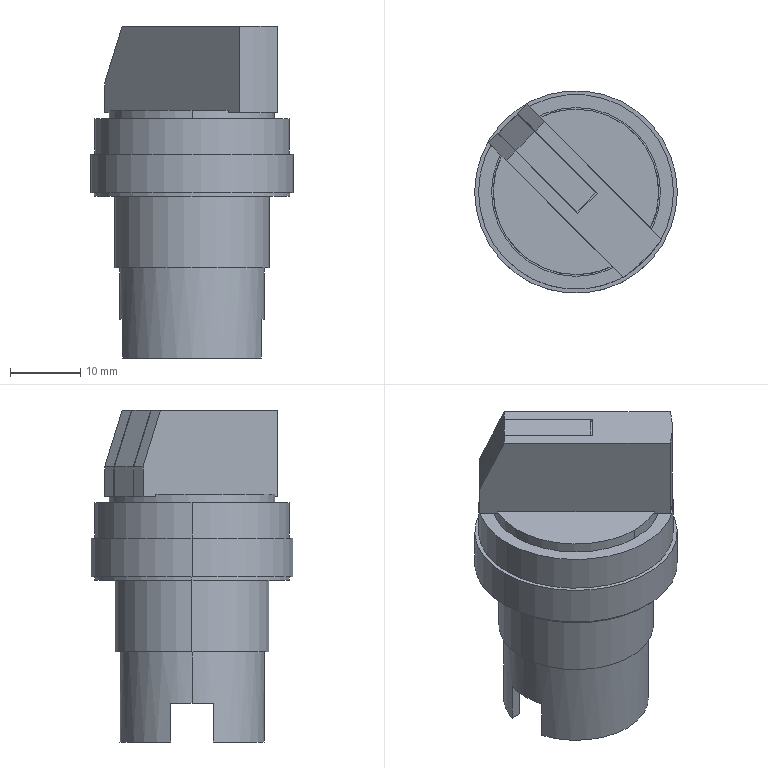Part | STEP file | A22NZ_2B[]_N[]A_BASE | 1 solid | 60 faces | box 28.8 x 28.8 x 47.2 mm | volume 14426 mm3 | plane 41 | cylinder 19 | commonest cylinder face diameters 13.2 x2 17.7 x2 20.6 x2 22 x2 23.5 x2 24 x2